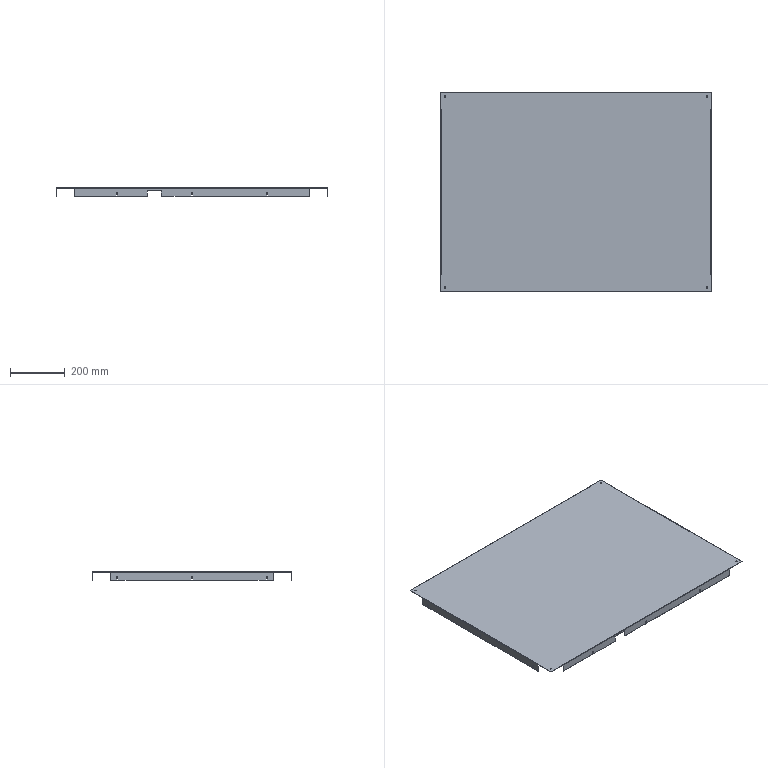Part | STEP file | Side seal plate large | 1 solid | 166 faces | box 988 x 728 x 30 mm | volume 958433 mm3 | plane 106 | cylinder 60 | commonest cylinder face diameters 4.5 x24 4 x20 5 x8 1.2 x4 3.6 x4